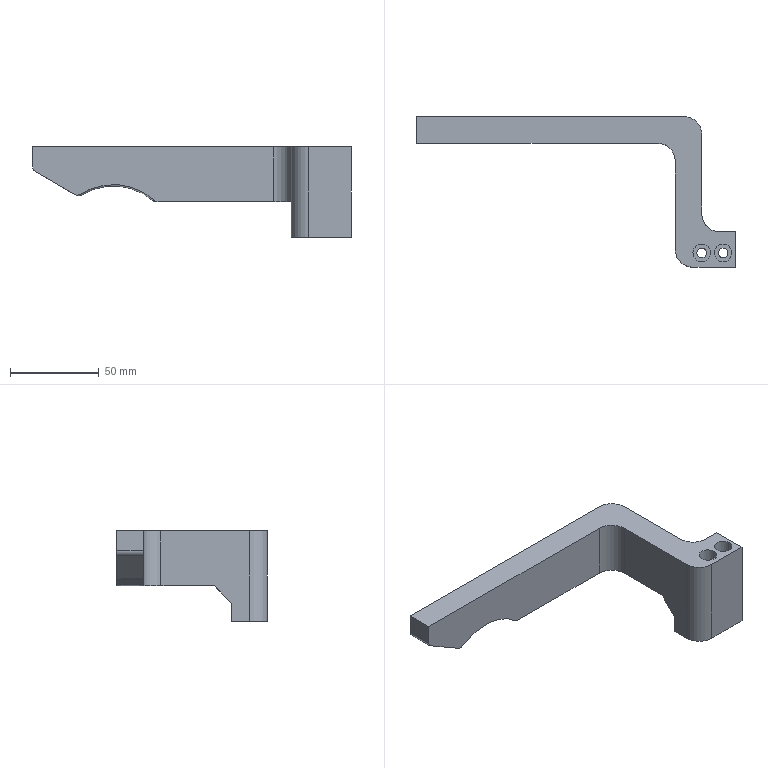NC program | NX | posted with a generic post | part box 180 x 85 x 51 mm
Lines 1 to 23 of 44959:
N10 G17 G21 G94 G90
(FLOOR_WALL , TOOL : D63)
N12 T01 M6
N14 G54
N16 G17 G0 G90 X129.5 Y-47.497 S6500 M3
N18 G43 Z30. H1
N20 Z3.
N22 G94 G1 Z0. F1500.
N24 X126.5
N26 X-126.5
N28 Y-35.381
N30 Y-12.599
N32 X126.5
N34 Y22.3
N36 X-126.5
N38 X-129.5
N40 Z3.
N42 G0 Z30.
N44 M5